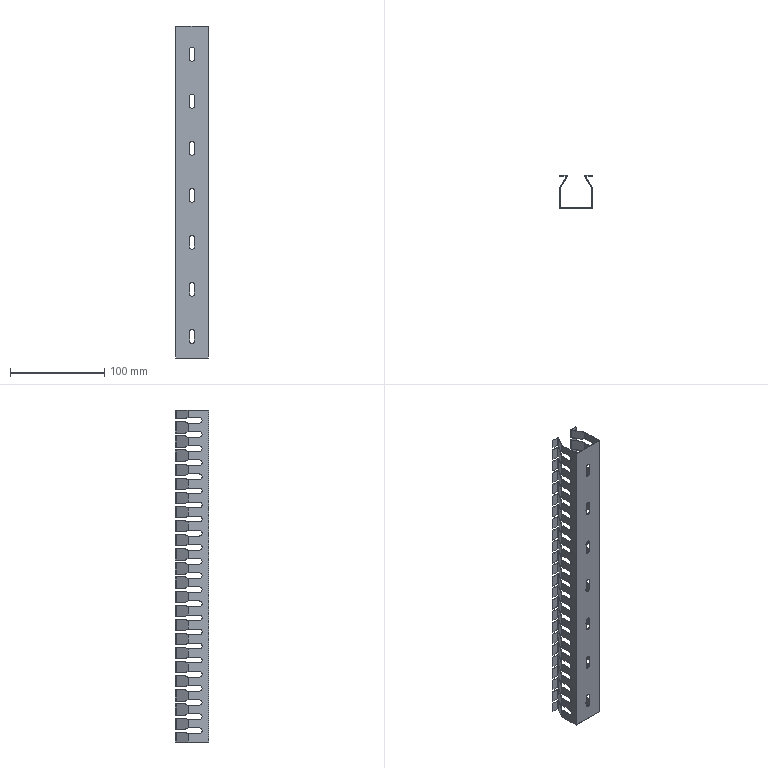Part | SolidWorks | features BaseBody 1, ICE 1 | 1 solid | 742 faces | box 35 x 35.5 x 353 mm | volume 17858 mm3 | plane 446 | cylinder 296 | commonest cylinder face diameters 6 x138 1 x72 2 x72 5 x14